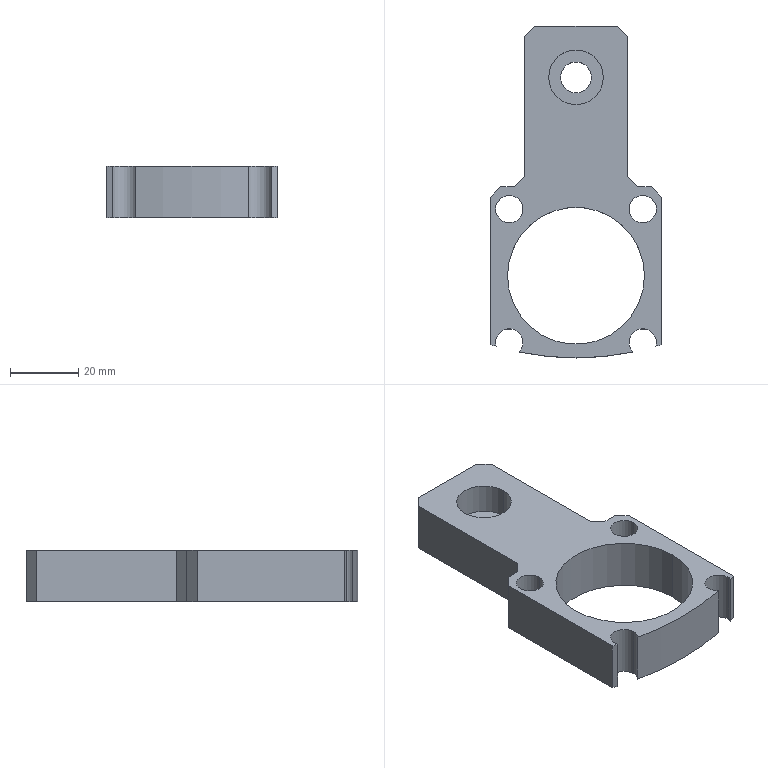Part | SolidWorks | features ICE 4, Chamfer 1, Cut 1, Extrusion 1 | 1 solid | 35 faces | box 50 x 97 x 15 mm | volume 33774 mm3 | cylinder 19 | plane 16 | commonest cylinder face diameters 8 x10 164 x3 9 x2 16 x2 40 x2
STEP:
#1=CARTESIAN_POINT('',(23.274,-3.814,15.));
#2=VERTEX_POINT('',#1);
#3=CARTESIAN_POINT('',(15.274,-3.814,15.));
#4=VERTEX_POINT('',#3);
#5=CARTESIAN_POINT('',(19.274,-3.814,15.));
#6=DIRECTION('',(0.,0.,-1.));
#7=DIRECTION('',(-1.,0.,0.));
#8=AXIS2_PLACEMENT_3D('',#5,#6,#7);
#9=CIRCLE('',#8,4.);
#10=EDGE_CURVE('',#2,#4,#9,.T.);
#11=ORIENTED_EDGE('',*,*,#10,.F.);
#12=CARTESIAN_POINT('',(23.274,-3.814,0.));
#13=VERTEX_POINT('',#12);
#14=CARTESIAN_POINT('',(23.274,-3.814,15.));
#15=DIRECTION('',(0.,0.,-1.));
#16=VECTOR('',#15,1000.);
#17=LINE('',#14,#16);
#18=EDGE_CURVE('',#2,#13,#17,.T.);
#19=ORIENTED_EDGE('',*,*,#18,.T.);
#20=CARTESIAN_POINT('',(15.274,-3.814,0.));
#21=VERTEX_POINT('',#20);
#22=CARTESIAN_POINT('',(19.274,-3.814,0.));
#23=DIRECTION('',(0.,0.,-1.));
#24=DIRECTION('',(-1.,0.,0.));
#25=AXIS2_PLACEMENT_3D('',#22,#23,#24);
#26=CIRCLE('',#25,4.);
#27=EDGE_CURVE('',#13,#21,#26,.T.);
#28=ORIENTED_EDGE('',*,*,#27,.T.);
#29=CARTESIAN_POINT('',(15.274,-3.814,15.));
#30=DIRECTION('',(0.,0.,-1.));
#31=VECTOR('',#30,1000.);
#32=LINE('',#29,#31);
#33=EDGE_CURVE('',#4,#21,#32,.T.);
#34=ORIENTED_EDGE('',*,*,#33,.F.);
#35=EDGE_LOOP('',(#11,#19,#28,#34));
#36=FACE_OUTER_BOUND('',#35,.T.);
#37=CARTESIAN_POINT('',(19.274,-3.814,15.));
#38=DIRECTION('',(0.,0.,-1.));
#39=DIRECTION('',(-1.,0.,0.));
#40=AXIS2_PLACEMENT_3D('',#37,#38,#39);
#41=CYLINDRICAL_SURFACE('',#40,4.);
#42=ADVANCED_FACE('',(#36),#41,.F.);
#43=CARTESIAN_POINT('',(-15.726,-3.814,15.));
#44=VERTEX_POINT('',#43);
#45=CARTESIAN_POINT('',(-23.726,-3.814,15.));
#46=VERTEX_POINT('',#45);
#47=CARTESIAN_POINT('',(-19.726,-3.814,15.));
#48=DIRECTION('',(0.,0.,-1.));
#49=DIRECTION('',(-1.,0.,0.));
#50=AXIS2_PLACEMENT_3D('',#47,#48,#49);
#51=CIRCLE('',#50,4.);
#52=EDGE_CURVE('',#44,#46,#51,.T.);
#53=ORIENTED_EDGE('',*,*,#52,.F.);
#54=CARTESIAN_POINT('',(-15.726,-3.814,0.));
#55=VERTEX_POINT('',#54);
#56=CARTESIAN_POINT('',(-15.726,-3.814,15.));
#57=DIRECTION('',(0.,0.,-1.));
#58=VECTOR('',#57,1000.);
#59=LINE('',#56,#58);
#60=EDGE_CURVE('',#44,#55,#59,.T.);
#61=ORIENTED_EDGE('',*,*,#60,.T.);
#62=CARTESIAN_POINT('',(-23.726,-3.814,0.));
#63=VERTEX_POINT('',#62);
#64=CARTESIAN_POINT('',(-19.726,-3.814,0.));
#65=DIRECTION('',(0.,0.,-1.));
#66=DIRECTION('',(-1.,0.,0.));
#67=AXIS2_PLACEMENT_3D('',#64,#65,#66);
#68=CIRCLE('',#67,4.);
#69=EDGE_CURVE('',#55,#63,#68,.T.);
#70=ORIENTED_EDGE('',*,*,#69,.T.);
#71=CARTESIAN_POINT('',(-23.726,-3.814,15.));
#72=DIRECTION('',(0.,0.,-1.));
#73=VECTOR('',#72,1000.);
#74=LINE('',#71,#73);
#75=EDGE_CURVE('',#46,#63,#74,.T.);
#76=ORIENTED_EDGE('',*,*,#75,.F.);
#77=EDGE_LOOP('',(#53,#61,#70,#76));
#78=FACE_OUTER_BOUND('',#77,.T.);
#79=CARTESIAN_POINT('',(-19.726,-3.814,15.));
#80=DIRECTION('',(0.,0.,-1.));
#81=DIRECTION('',(-1.,0.,0.));
#82=AXIS2_PLACEMENT_3D('',#79,#80,#81);
#83=CYLINDRICAL_SURFACE('',#82,4.);
#84=ADVANCED_FACE('',(#78),#83,.F.);
#85=CARTESIAN_POINT('',(19.774,-23.314,15.));
#86=VERTEX_POINT('',#85);
#87=CARTESIAN_POINT('',(-20.226,-23.314,15.));
#88=VERTEX_POINT('',#87);
#89=CARTESIAN_POINT('',(-0.2255,-23.314,15.));
#90=DIRECTION('',(0.,0.,-1.));
#91=DIRECTION('',(-1.,0.,0.));
#92=AXIS2_PLACEMENT_3D('',#89,#90,#91);
#93=CIRCLE('',#92,20.);
#94=EDGE_CURVE('',#86,#88,#93,.T.);
#95=ORIENTED_EDGE('',*,*,#94,.F.);
#96=CARTESIAN_POINT('',(19.774,-23.314,0.));
#97=VERTEX_POINT('',#96);
#98=CARTESIAN_POINT('',(19.774,-23.314,15.));
#99=DIRECTION('',(0.,0.,-1.));
#100=VECTOR('',#99,1000.);
#101=LINE('',#98,#100);
#102=EDGE_CURVE('',#86,#97,#101,.T.);
#103=ORIENTED_EDGE('',*,*,#102,.T.);
#104=CARTESIAN_POINT('',(-20.226,-23.314,0.));
#105=VERTEX_POINT('',#104);
#106=CARTESIAN_POINT('',(-0.2255,-23.314,0.));
#107=DIRECTION('',(0.,0.,-1.));
#108=DIRECTION('',(-1.,0.,0.));
#109=AXIS2_PLACEMENT_3D('',#106,#107,#108);
#110=CIRCLE('',#109,20.);
#111=EDGE_CURVE('',#97,#105,#110,.T.);
#112=ORIENTED_EDGE('',*,*,#111,.T.);
#113=CARTESIAN_POINT('',(-20.226,-23.314,15.));
#114=DIRECTION('',(0.,0.,-1.));
#115=VECTOR('',#114,1000.);
#116=LINE('',#113,#115);
#117=EDGE_CURVE('',#88,#105,#116,.T.);
#118=ORIENTED_EDGE('',*,*,#117,.F.);
#119=EDGE_LOOP('',(#95,#103,#112,#118));
#120=FACE_OUTER_BOUND('',#119,.T.);
#121=CARTESIAN_POINT('',(-0.2255,-23.314,15.));
#122=DIRECTION('',(0.,0.,-1.));
#123=DIRECTION('',(-1.,0.,0.));
#124=AXIS2_PLACEMENT_3D('',#121,#122,#123);
#125=CYLINDRICAL_SURFACE('',#124,20.);
#126=ADVANCED_FACE('',(#120),#125,.F.);
#127=CARTESIAN_POINT('',(-4.726,34.686,0.));
#128=VERTEX_POINT('',#127);
#129=CARTESIAN_POINT('',(4.274,34.686,0.));
#130=VERTEX_POINT('',#129);
#131=CARTESIAN_POINT('',(-0.2255,34.686,0.));
#132=DIRECTION('',(0.,0.,1.));
#133=DIRECTION('',(1.,0.,0.));
#134=AXIS2_PLACEMENT_3D('',#131,#132,#133);
#135=CIRCLE('',#134,4.5);
#136=EDGE_CURVE('',#128,#130,#135,.T.);
#137=ORIENTED_EDGE('',*,*,#136,.F.);
#138=CARTESIAN_POINT('',(-4.726,34.686,6.));
#139=VERTEX_POINT('',#138);
#140=CARTESIAN_POINT('',(-4.726,34.686,0.));
#141=DIRECTION('',(0.,0.,1.));
#142=VECTOR('',#141,1000.);
#143=LINE('',#140,#142);
#144=EDGE_CURVE('',#128,#139,#143,.T.);
#145=ORIENTED_EDGE('',*,*,#144,.T.);
#146=CARTESIAN_POINT('',(4.274,34.686,6.));
#147=VERTEX_POINT('',#146);
#148=CARTESIAN_POINT('',(-0.2255,34.686,6.));
#149=DIRECTION('',(0.,0.,1.));
#150=DIRECTION('',(1.,0.,0.));
#151=AXIS2_PLACEMENT_3D('',#148,#149,#150);
#152=CIRCLE('',#151,4.5);
#153=EDGE_CURVE('',#139,#147,#152,.T.);
#154=ORIENTED_EDGE('',*,*,#153,.T.);
#155=CARTESIAN_POINT('',(4.274,34.686,0.));
#156=DIRECTION('',(0.,0.,1.));
#157=VECTOR('',#156,1000.);
#158=LINE('',#155,#157);
#159=EDGE_CURVE('',#130,#147,#158,.T.);
#160=ORIENTED_EDGE('',*,*,#159,.F.);
#161=EDGE_LOOP('',(#137,#145,#154,#160));
#162=FACE_OUTER_BOUND('',#161,.T.);
#163=CARTESIAN_POINT('',(-0.2255,34.686,0.));
#164=DIRECTION('',(0.,0.,1.));
#165=DIRECTION('',(1.,0.,0.));
#166=AXIS2_PLACEMENT_3D('',#163,#164,#165);
#167=CYLINDRICAL_SURFACE('',#166,4.5);
#168=ADVANCED_FACE('',(#162),#167,.F.);
#169=CARTESIAN_POINT('',(-8.226,34.686,6.));
#170=VERTEX_POINT('',#169);
#171=CARTESIAN_POINT('',(7.774,34.686,6.));
#172=VERTEX_POINT('',#171);
#173=CARTESIAN_POINT('',(-0.2255,34.686,6.));
#174=DIRECTION('',(0.,0.,1.));
#175=DIRECTION('',(1.,0.,0.));
#176=AXIS2_PLACEMENT_3D('',#173,#174,#175);
#177=CIRCLE('',#176,8.);
#178=EDGE_CURVE('',#170,#172,#177,.T.);
#179=ORIENTED_EDGE('',*,*,#178,.F.);
#180=CARTESIAN_POINT('',(-8.226,34.686,15.));
#181=VERTEX_POINT('',#180);
#182=CARTESIAN_POINT('',(-8.226,34.686,6.));
#183=DIRECTION('',(0.,0.,1.));
#184=VECTOR('',#183,1000.);
#185=LINE('',#182,#184);
#186=EDGE_CURVE('',#170,#181,#185,.T.);
#187=ORIENTED_EDGE('',*,*,#186,.T.);
#188=CARTESIAN_POINT('',(7.774,34.686,15.));
#189=VERTEX_POINT('',#188);
#190=CARTESIAN_POINT('',(-0.2255,34.686,15.));
#191=DIRECTION('',(0.,0.,1.));
#192=DIRECTION('',(1.,0.,0.));
#193=AXIS2_PLACEMENT_3D('',#190,#191,#192);
#194=CIRCLE('',#193,8.);
#195=EDGE_CURVE('',#181,#189,#194,.T.);
#196=ORIENTED_EDGE('',*,*,#195,.T.);
#197=CARTESIAN_POINT('',(7.774,34.686,6.));
#198=DIRECTION('',(0.,0.,1.));
#199=VECTOR('',#198,1000.);
#200=LINE('',#197,#199);
#201=EDGE_CURVE('',#172,#189,#200,.T.);
#202=ORIENTED_EDGE('',*,*,#201,.F.);
#203=EDGE_LOOP('',(#179,#187,#196,#202));
#204=FACE_OUTER_BOUND('',#203,.T.);
#205=CARTESIAN_POINT('',(-0.2255,34.686,6.));
#206=DIRECTION('',(0.,0.,1.));
#207=DIRECTION('',(1.,0.,0.));
#208=AXIS2_PLACEMENT_3D('',#205,#206,#207);
#209=CYLINDRICAL_SURFACE('',#208,8.);
#210=ADVANCED_FACE('',(#204),#209,.F.);
#211=CARTESIAN_POINT('',(23.274,-42.814,15.));
#212=VERTEX_POINT('',#211);
#213=CARTESIAN_POINT('',(23.118,-43.922,15.));
#214=VERTEX_POINT('',#213);
#215=CARTESIAN_POINT('',(19.274,-42.814,15.));
#216=DIRECTION('',(0.,0.,-1.));
#217=DIRECTION('',(-1.,0.,0.));
#218=AXIS2_PLACEMENT_3D('',#215,#216,#217);
#219=CIRCLE('',#218,4.);
#220=EDGE_CURVE('',#212,#214,#219,.T.);
#221=ORIENTED_EDGE('',*,*,#220,.F.);
#222=CARTESIAN_POINT('',(23.274,-42.814,0.));
#223=VERTEX_POINT('',#222);
#224=CARTESIAN_POINT('',(23.274,-42.814,15.));
#225=DIRECTION('',(0.,0.,-1.));
#226=VECTOR('',#225,1000.);
#227=LINE('',#224,#226);
#228=EDGE_CURVE('',#212,#223,#227,.T.);
#229=ORIENTED_EDGE('',*,*,#228,.T.);
#230=CARTESIAN_POINT('',(23.118,-43.922,0.));
#231=VERTEX_POINT('',#230);
#232=CARTESIAN_POINT('',(19.274,-42.814,0.));
#233=DIRECTION('',(0.,0.,-1.));
#234=DIRECTION('',(-1.,0.,0.));
#235=AXIS2_PLACEMENT_3D('',#232,#233,#234);
#236=CIRCLE('',#235,4.);
#237=EDGE_CURVE('',#223,#231,#236,.T.);
#238=ORIENTED_EDGE('',*,*,#237,.T.);
#239=CARTESIAN_POINT('',(23.118,-43.922,7.5));
#240=DIRECTION('',(0.,0.,-1.));
#241=VECTOR('',#240,1000.);
#242=LINE('',#239,#241);
#243=EDGE_CURVE('',#214,#231,#242,.T.);
#244=ORIENTED_EDGE('',*,*,#243,.F.);
#245=EDGE_LOOP('',(#221,#229,#238,#244));
#246=FACE_OUTER_BOUND('',#245,.T.);
#247=CARTESIAN_POINT('',(19.274,-42.814,15.));
#248=DIRECTION('',(0.,0.,-1.));
#249=DIRECTION('',(-1.,0.,0.));
#250=AXIS2_PLACEMENT_3D('',#247,#248,#249);
#251=CYLINDRICAL_SURFACE('',#250,4.);
#252=ADVANCED_FACE('',(#246),#251,.F.);
#253=ORIENTED_EDGE('',*,*,#228,.F.);
#254=CARTESIAN_POINT('',(15.274,-42.814,15.));
#255=VERTEX_POINT('',#254);
#256=CARTESIAN_POINT('',(19.274,-42.814,15.));
#257=DIRECTION('',(0.,0.,-1.));
#258=DIRECTION('',(-1.,0.,0.));
#259=AXIS2_PLACEMENT_3D('',#256,#257,#258);
#260=CIRCLE('',#259,4.);
#261=EDGE_CURVE('',#255,#212,#260,.T.);
#262=ORIENTED_EDGE('',*,*,#261,.F.);
#263=CARTESIAN_POINT('',(15.274,-42.814,0.));
#264=VERTEX_POINT('',#263);
#265=CARTESIAN_POINT('',(15.274,-42.814,15.));
#266=DIRECTION('',(0.,0.,-1.));
#267=VECTOR('',#266,1000.);
#268=LINE('',#265,#267);
#269=EDGE_CURVE('',#255,#264,#268,.T.);
#270=ORIENTED_EDGE('',*,*,#269,.T.);
#271=CARTESIAN_POINT('',(19.274,-42.814,0.));
#272=DIRECTION('',(0.,0.,-1.));
#273=DIRECTION('',(-1.,0.,0.));
#274=AXIS2_PLACEMENT_3D('',#271,#272,#273);
#275=CIRCLE('',#274,4.);
#276=EDGE_CURVE('',#264,#223,#275,.T.);
#277=ORIENTED_EDGE('',*,*,#276,.T.);
#278=EDGE_LOOP('',(#253,#262,#270,#277));
#279=FACE_OUTER_BOUND('',#278,.T.);
#280=CARTESIAN_POINT('',(19.274,-42.814,15.));
#281=DIRECTION('',(0.,0.,-1.));
#282=DIRECTION('',(-1.,0.,0.));
#283=AXIS2_PLACEMENT_3D('',#280,#281,#282);
#284=CYLINDRICAL_SURFACE('',#283,4.);
#285=ADVANCED_FACE('',(#279),#284,.F.);
#286=CARTESIAN_POINT('',(-15.726,-42.814,15.));
#287=VERTEX_POINT('',#286);
#288=CARTESIAN_POINT('',(-16.863,-45.609,15.));
#289=VERTEX_POINT('',#288);
#290=CARTESIAN_POINT('',(-19.726,-42.814,15.));
#291=DIRECTION('',(0.,0.,-1.));
#292=DIRECTION('',(-1.,0.,0.));
#293=AXIS2_PLACEMENT_3D('',#290,#291,#292);
#294=CIRCLE('',#293,4.);
#295=EDGE_CURVE('',#287,#289,#294,.T.);
#296=ORIENTED_EDGE('',*,*,#295,.F.);
#297=CARTESIAN_POINT('',(-15.726,-42.814,0.));
#298=VERTEX_POINT('',#297);
#299=CARTESIAN_POINT('',(-15.726,-42.814,15.));
#300=DIRECTION('',(0.,0.,-1.));
#301=VECTOR('',#300,1000.);
#302=LINE('',#299,#301);
#303=EDGE_CURVE('',#287,#298,#302,.T.);
#304=ORIENTED_EDGE('',*,*,#303,.T.);
#305=CARTESIAN_POINT('',(-16.863,-45.609,0.));
#306=VERTEX_POINT('',#305);
#307=CARTESIAN_POINT('',(-19.726,-42.814,0.));
#308=DIRECTION('',(0.,0.,-1.));
#309=DIRECTION('',(-1.,0.,0.));
#310=AXIS2_PLACEMENT_3D('',#307,#308,#309);
#311=CIRCLE('',#310,4.);
#312=EDGE_CURVE('',#298,#306,#311,.T.);
#313=ORIENTED_EDGE('',*,*,#312,.T.);
#314=CARTESIAN_POINT('',(-16.863,-45.609,7.5));
#315=DIRECTION('',(0.,0.,-1.));
#316=VECTOR('',#315,1000.);
#317=LINE('',#314,#316);
#318=EDGE_CURVE('',#289,#306,#317,.T.);
#319=ORIENTED_EDGE('',*,*,#318,.F.);
#320=EDGE_LOOP('',(#296,#304,#313,#319));
#321=FACE_OUTER_BOUND('',#320,.T.);
#322=CARTESIAN_POINT('',(-19.726,-42.814,15.));
#323=DIRECTION('',(0.,0.,-1.));
#324=DIRECTION('',(-1.,0.,0.));
#325=AXIS2_PLACEMENT_3D('',#322,#323,#324);
#326=CYLINDRICAL_SURFACE('',#325,4.);
#327=ADVANCED_FACE('',(#321),#326,.F.);
#328=ORIENTED_EDGE('',*,*,#303,.F.);
#329=CARTESIAN_POINT('',(-23.726,-42.814,15.));
#330=VERTEX_POINT('',#329);
#331=CARTESIAN_POINT('',(-19.726,-42.814,15.));
#332=DIRECTION('',(0.,0.,-1.));
#333=DIRECTION('',(-1.,0.,0.));
#334=AXIS2_PLACEMENT_3D('',#331,#332,#333);
#335=CIRCLE('',#334,4.);
#336=EDGE_CURVE('',#330,#287,#335,.T.);
#337=ORIENTED_EDGE('',*,*,#336,.F.);
#338=CARTESIAN_POINT('',(-23.726,-42.814,0.));
#339=VERTEX_POINT('',#338);
#340=CARTESIAN_POINT('',(-23.726,-42.814,15.));
#341=DIRECTION('',(0.,0.,-1.));
#342=VECTOR('',#341,1000.);
#343=LINE('',#340,#342);
#344=EDGE_CURVE('',#330,#339,#343,.T.);
#345=ORIENTED_EDGE('',*,*,#344,.T.);
#346=CARTESIAN_POINT('',(-19.726,-42.814,0.));
#347=DIRECTION('',(0.,0.,-1.));
#348=DIRECTION('',(-1.,0.,0.));
#349=AXIS2_PLACEMENT_3D('',#346,#347,#348);
#350=CIRCLE('',#349,4.);
#351=EDGE_CURVE('',#339,#298,#350,.T.);
#352=ORIENTED_EDGE('',*,*,#351,.T.);
#353=EDGE_LOOP('',(#328,#337,#345,#352));
#354=FACE_OUTER_BOUND('',#353,.T.);
#355=CARTESIAN_POINT('',(-19.726,-42.814,15.));
#356=DIRECTION('',(0.,0.,-1.));
#357=DIRECTION('',(-1.,0.,0.));
#358=AXIS2_PLACEMENT_3D('',#355,#356,#357);
#359=CYLINDRICAL_SURFACE('',#358,4.);
#360=ADVANCED_FACE('',(#354),#359,.F.);
#361=CARTESIAN_POINT('',(-25.226,-43.411,15.));
#362=VERTEX_POINT('',#361);
#363=CARTESIAN_POINT('',(-25.226,-43.411,0.));
#364=VERTEX_POINT('',#363);
#365=CARTESIAN_POINT('',(-25.226,-43.411,15.));
#366=DIRECTION('',(0.,0.,-1.));
#367=VECTOR('',#366,1000.);
#368=LINE('',#365,#367);
#369=EDGE_CURVE('',#362,#364,#368,.T.);
#370=ORIENTED_EDGE('',*,*,#369,.F.);
#371=CARTESIAN_POINT('',(-25.226,-0.3145,15.));
#372=VERTEX_POINT('',#371);
#373=CARTESIAN_POINT('',(-25.226,49.686,15.));
#374=DIRECTION('',(0.,-1.,0.));
#375=VECTOR('',#374,1000.);
#376=LINE('',#373,#375);
#377=EDGE_CURVE('',#372,#362,#376,.T.);
#378=ORIENTED_EDGE('',*,*,#377,.F.);
#379=CARTESIAN_POINT('',(-25.226,-0.3145,0.));
#380=VERTEX_POINT('',#379);
#381=CARTESIAN_POINT('',(-25.226,-0.3145,15.));
#382=DIRECTION('',(0.,0.,-1.));
#383=VECTOR('',#382,1000.);
#384=LINE('',#381,#383);
#385=EDGE_CURVE('',#372,#380,#384,.T.);
#386=ORIENTED_EDGE('',*,*,#385,.T.);
#387=CARTESIAN_POINT('',(-25.226,49.686,0.));
#388=DIRECTION('',(0.,-1.,0.));
#389=VECTOR('',#388,1000.);
#390=LINE('',#387,#389);
#391=EDGE_CURVE('',#380,#364,#390,.T.);
#392=ORIENTED_EDGE('',*,*,#391,.T.);
#393=EDGE_LOOP('',(#370,#378,#386,#392));
#394=FACE_OUTER_BOUND('',#393,.T.);
#395=CARTESIAN_POINT('',(-25.226,49.686,15.));
#396=DIRECTION('',(1.,0.,0.));
#397=DIRECTION('',(0.,1.,0.));
#398=AXIS2_PLACEMENT_3D('',#395,#396,#397);
#399=PLANE('',#398);
#400=ADVANCED_FACE('',(#394),#399,.F.);
#401=CARTESIAN_POINT('',(24.774,-43.411,0.));
#402=VERTEX_POINT('',#401);
#403=CARTESIAN_POINT('',(24.774,-43.411,15.));
#404=VERTEX_POINT('',#403);
#405=CARTESIAN_POINT('',(24.774,-43.411,15.));
#406=DIRECTION('',(0.,0.,1.));
#407=VECTOR('',#406,1000.);
#408=LINE('',#405,#407);
#409=EDGE_CURVE('',#402,#404,#408,.T.);
#410=ORIENTED_EDGE('',*,*,#409,.F.);
#411=CARTESIAN_POINT('',(24.774,-0.3145,0.));
#412=VERTEX_POINT('',#411);
#413=CARTESIAN_POINT('',(24.774,49.686,0.));
#414=DIRECTION('',(0.,1.,0.));
#415=VECTOR('',#414,1000.);
#416=LINE('',#413,#415);
#417=EDGE_CURVE('',#402,#412,#416,.T.);
#418=ORIENTED_EDGE('',*,*,#417,.T.);
#419=CARTESIAN_POINT('',(24.774,-0.3145,15.));
#420=VERTEX_POINT('',#419);
#421=CARTESIAN_POINT('',(24.774,-0.3145,15.));
#422=DIRECTION('',(0.,0.,1.));
#423=VECTOR('',#422,1000.);
#424=LINE('',#421,#423);
#425=EDGE_CURVE('',#412,#420,#424,.T.);
#426=ORIENTED_EDGE('',*,*,#425,.T.);
#427=CARTESIAN_POINT('',(24.774,49.686,15.));
#428=DIRECTION('',(0.,1.,0.));
#429=VECTOR('',#428,1000.);
#430=LINE('',#427,#429);
#431=EDGE_CURVE('',#404,#420,#430,.T.);
#432=ORIENTED_EDGE('',*,*,#431,.F.);
#433=EDGE_LOOP('',(#410,#418,#426,#432));
#434=FACE_OUTER_BOUND('',#433,.T.);
#435=CARTESIAN_POINT('',(24.774,49.686,15.));
#436=DIRECTION('',(-1.,0.,0.));
#437=DIRECTION('',(0.,-1.,0.));
#438=AXIS2_PLACEMENT_3D('',#435,#436,#437);
#439=PLANE('',#438);
#440=ADVANCED_FACE('',(#434),#439,.F.);
#441=CARTESIAN_POINT('',(19.274,-3.814,15.));
#442=DIRECTION('',(0.,0.,-1.));
#443=DIRECTION('',(-1.,0.,0.));
#444=AXIS2_PLACEMENT_3D('',#441,#442,#443);
#445=CIRCLE('',#444,4.);
#446=EDGE_CURVE('',#4,#2,#445,.T.);
#447=ORIENTED_EDGE('',*,*,#446,.T.);
#448=ORIENTED_EDGE('',*,*,#10,.T.);
#449=EDGE_LOOP('',(#447,#448));
#450=FACE_BOUND('',#449,.T.);
#451=CARTESIAN_POINT('',(-19.726,-3.814,15.));
#452=DIRECTION('',(0.,0.,-1.));
#453=DIRECTION('',(-1.,0.,0.));
#454=AXIS2_PLACEMENT_3D('',#451,#452,#453);
#455=CIRCLE('',#454,4.);
#456=EDGE_CURVE('',#46,#44,#455,.T.);
#457=ORIENTED_EDGE('',*,*,#456,.T.);
#458=ORIENTED_EDGE('',*,*,#52,.T.);
#459=EDGE_LOOP('',(#457,#458));
#460=FACE_BOUND('',#459,.T.);
#461=CARTESIAN_POINT('',(-0.2255,-23.314,15.));
#462=DIRECTION('',(0.,0.,-1.));
#463=DIRECTION('',(-1.,0.,0.));
#464=AXIS2_PLACEMENT_3D('',#461,#462,#463);
#465=CIRCLE('',#464,20.);
#466=EDGE_CURVE('',#88,#86,#465,.T.);
#467=ORIENTED_EDGE('',*,*,#466,.T.);
#468=ORIENTED_EDGE('',*,*,#94,.T.);
#469=EDGE_LOOP('',(#467,#468));
#470=FACE_BOUND('',#469,.T.);
#471=CARTESIAN_POINT('',(-0.2255,34.686,15.));
#472=DIRECTION('',(0.,0.,1.));
#473=DIRECTION('',(1.,0.,0.));
#474=AXIS2_PLACEMENT_3D('',#471,#472,#473);
#475=CIRCLE('',#474,8.);
#476=EDGE_CURVE('',#189,#181,#475,.T.);
#477=ORIENTED_EDGE('',*,*,#476,.F.);
#478=ORIENTED_EDGE('',*,*,#195,.F.);
#479=EDGE_LOOP('',(#477,#478));
#480=FACE_BOUND('',#479,.T.);
#481=ORIENTED_EDGE('',*,*,#377,.T.);
#482=CARTESIAN_POINT('',(-23.569,-43.922,15.));
#483=VERTEX_POINT('',#482);
#484=CARTESIAN_POINT('',(-0.2255,34.686,15.));
#485=DIRECTION('',(0.,0.,-1.));
#486=DIRECTION('',(-1.,0.,0.));
#487=AXIS2_PLACEMENT_3D('',#484,#485,#486);
#488=CIRCLE('',#487,82.);
#489=EDGE_CURVE('',#483,#362,#488,.T.);
#490=ORIENTED_EDGE('',*,*,#489,.F.);
#491=CARTESIAN_POINT('',(-19.726,-42.814,15.));
#492=DIRECTION('',(0.,0.,-1.));
#493=DIRECTION('',(-1.,0.,0.));
#494=AXIS2_PLACEMENT_3D('',#491,#492,#493);
#495=CIRCLE('',#494,4.);
#496=EDGE_CURVE('',#483,#330,#495,.T.);
#497=ORIENTED_EDGE('',*,*,#496,.T.);
#498=ORIENTED_EDGE('',*,*,#336,.T.);
#499=ORIENTED_EDGE('',*,*,#295,.T.);
#500=CARTESIAN_POINT('',(16.412,-45.609,15.));
#501=VERTEX_POINT('',#500);
#502=CARTESIAN_POINT('',(-0.2255,34.686,15.));
#503=DIRECTION('',(0.,0.,-1.));
#504=DIRECTION('',(-1.,0.,0.));
#505=AXIS2_PLACEMENT_3D('',#502,#503,#504);
#506=CIRCLE('',#505,82.);
#507=EDGE_CURVE('',#501,#289,#506,.T.);
#508=ORIENTED_EDGE('',*,*,#507,.F.);
#509=CARTESIAN_POINT('',(19.274,-42.814,15.));
#510=DIRECTION('',(0.,0.,-1.));
#511=DIRECTION('',(-1.,0.,0.));
#512=AXIS2_PLACEMENT_3D('',#509,#510,#511);
#513=CIRCLE('',#512,4.);
#514=EDGE_CURVE('',#501,#255,#513,.T.);
#515=ORIENTED_EDGE('',*,*,#514,.T.);
#516=ORIENTED_EDGE('',*,*,#261,.T.);
#517=ORIENTED_EDGE('',*,*,#220,.T.);
#518=CARTESIAN_POINT('',(-0.2255,34.686,15.));
#519=DIRECTION('',(0.,0.,-1.));
#520=DIRECTION('',(-1.,0.,0.));
#521=AXIS2_PLACEMENT_3D('',#518,#519,#520);
#522=CIRCLE('',#521,82.);
#523=EDGE_CURVE('',#404,#214,#522,.T.);
#524=ORIENTED_EDGE('',*,*,#523,.F.);
#525=ORIENTED_EDGE('',*,*,#431,.T.);
#526=CARTESIAN_POINT('',(21.774,2.686,15.));
#527=VERTEX_POINT('',#526);
#528=CARTESIAN_POINT('',(12.23,12.23,15.));
#529=DIRECTION('',(-0.7071,0.7071,0.));
#530=VECTOR('',#529,1000.);
#531=LINE('',#528,#530);
#532=EDGE_CURVE('',#420,#527,#531,.T.);
#533=ORIENTED_EDGE('',*,*,#532,.T.);
#534=CARTESIAN_POINT('',(17.774,2.686,15.));
#535=VERTEX_POINT('',#534);
#536=CARTESIAN_POINT('',(14.774,2.686,15.));
#537=DIRECTION('',(1.,0.,0.));
#538=VECTOR('',#537,1000.);
#539=LINE('',#536,#538);
#540=EDGE_CURVE('',#535,#527,#539,.T.);
#541=ORIENTED_EDGE('',*,*,#540,.F.);
#542=CARTESIAN_POINT('',(14.774,5.686,15.));
#543=VERTEX_POINT('',#542);
#544=CARTESIAN_POINT('',(17.774,2.686,15.));
#545=DIRECTION('',(-0.7071,0.7071,0.));
#546=VECTOR('',#545,1000.);
#547=LINE('',#544,#546);
#548=EDGE_CURVE('',#535,#543,#547,.T.);
#549=ORIENTED_EDGE('',*,*,#548,.T.);
#550=CARTESIAN_POINT('',(14.774,46.686,15.));
#551=VERTEX_POINT('',#550);
#552=CARTESIAN_POINT('',(14.774,64.722,15.));
#553=DIRECTION('',(0.,-1.,0.));
#554=VECTOR('',#553,1000.);
#555=LINE('',#552,#554);
#556=EDGE_CURVE('',#551,#543,#555,.T.);
#557=ORIENTED_EDGE('',*,*,#556,.F.);
#558=CARTESIAN_POINT('',(11.774,49.686,15.));
#559=VERTEX_POINT('',#558);
#560=CARTESIAN_POINT('',(30.73,30.73,15.));
#561=DIRECTION('',(-0.7071,0.7071,0.));
#562=VECTOR('',#561,1000.);
#563=LINE('',#560,#562);
#564=EDGE_CURVE('',#551,#559,#563,.T.);
#565=ORIENTED_EDGE('',*,*,#564,.T.);
#566=CARTESIAN_POINT('',(-12.226,49.686,15.));
#567=VERTEX_POINT('',#566);
#568=CARTESIAN_POINT('',(-25.226,49.686,15.));
#569=DIRECTION('',(-1.,0.,0.));
#570=VECTOR('',#569,1000.);
#571=LINE('',#568,#570);
#572=EDGE_CURVE('',#559,#567,#571,.T.);
#573=ORIENTED_EDGE('',*,*,#572,.T.);
#574=CARTESIAN_POINT('',(-15.226,46.686,15.));
#575=VERTEX_POINT('',#574);
#576=CARTESIAN_POINT('',(-30.956,30.956,15.));
#577=DIRECTION('',(-0.7071,-0.7071,0.));
#578=VECTOR('',#577,1000.);
#579=LINE('',#576,#578);
#580=EDGE_CURVE('',#567,#575,#579,.T.);
#581=ORIENTED_EDGE('',*,*,#580,.T.);
#582=CARTESIAN_POINT('',(-15.226,5.686,15.));
#583=VERTEX_POINT('',#582);
#584=CARTESIAN_POINT('',(-15.226,55.257,15.));
#585=DIRECTION('',(0.,1.,0.));
#586=VECTOR('',#585,1000.);
#587=LINE('',#584,#586);
#588=EDGE_CURVE('',#583,#575,#587,.T.);
#589=ORIENTED_EDGE('',*,*,#588,.F.);
#590=CARTESIAN_POINT('',(-18.226,2.686,15.));
#591=VERTEX_POINT('',#590);
#592=CARTESIAN_POINT('',(-15.226,5.686,15.));
#593=DIRECTION('',(-0.7071,-0.7071,0.));
#594=VECTOR('',#593,1000.);
#595=LINE('',#592,#594);
#596=EDGE_CURVE('',#583,#591,#595,.T.);
#597=ORIENTED_EDGE('',*,*,#596,.T.);
#598=CARTESIAN_POINT('',(-22.226,2.686,15.));
#599=VERTEX_POINT('',#598);
#600=CARTESIAN_POINT('',(-15.226,2.686,15.));
#601=DIRECTION('',(1.,0.,0.));
#602=VECTOR('',#601,1000.);
#603=LINE('',#600,#602);
#604=EDGE_CURVE('',#599,#591,#603,.T.);
#605=ORIENTED_EDGE('',*,*,#604,.F.);
#606=CARTESIAN_POINT('',(-12.456,12.456,15.));
#607=DIRECTION('',(-0.7071,-0.7071,0.));
#608=VECTOR('',#607,1000.);
#609=LINE('',#606,#608);
#610=EDGE_CURVE('',#599,#372,#609,.T.);
#611=ORIENTED_EDGE('',*,*,#610,.T.);
#612=EDGE_LOOP('',(#481,#490,#497,#498,#499,#508,#515,#516,#517,#524,#525,#533,#541,#549,#557,#565,#573,#581,#589,#597,#605,#611));
#613=FACE_OUTER_BOUND('',#612,.T.);
#614=CARTESIAN_POINT('',(0.,0.,15.));
#615=DIRECTION('',(0.,0.,1.));
#616=DIRECTION('',(1.,0.,0.));
#617=AXIS2_PLACEMENT_3D('',#614,#615,#616);
#618=PLANE('',#617);
#619=ADVANCED_FACE('',(#450,#460,#470,#480,#613),#618,.T.);
#620=CARTESIAN_POINT('',(19.274,-3.814,0.));
#621=DIRECTION('',(0.,0.,-1.));
#622=DIRECTION('',(-1.,0.,0.));
#623=AXIS2_PLACEMENT_3D('',#620,#621,#622);
#624=CIRCLE('',#623,4.);
#625=EDGE_CURVE('',#21,#13,#624,.T.);
#626=ORIENTED_EDGE('',*,*,#625,.F.);
#627=ORIENTED_EDGE('',*,*,#27,.F.);
#628=EDGE_LOOP('',(#626,#627));
#629=FACE_BOUND('',#628,.T.);
#630=CARTESIAN_POINT('',(-19.726,-3.814,0.));
#631=DIRECTION('',(0.,0.,-1.));
#632=DIRECTION('',(-1.,0.,0.));
#633=AXIS2_PLACEMENT_3D('',#630,#631,#632);
#634=CIRCLE('',#633,4.);
#635=EDGE_CURVE('',#63,#55,#634,.T.);
#636=ORIENTED_EDGE('',*,*,#635,.F.);
#637=ORIENTED_EDGE('',*,*,#69,.F.);
#638=EDGE_LOOP('',(#636,#637));
#639=FACE_BOUND('',#638,.T.);
#640=CARTESIAN_POINT('',(-0.2255,-23.314,0.));
#641=DIRECTION('',(0.,0.,-1.));
#642=DIRECTION('',(-1.,0.,0.));
#643=AXIS2_PLACEMENT_3D('',#640,#641,#642);
#644=CIRCLE('',#643,20.);
#645=EDGE_CURVE('',#105,#97,#644,.T.);
#646=ORIENTED_EDGE('',*,*,#645,.F.);
#647=ORIENTED_EDGE('',*,*,#111,.F.);
#648=EDGE_LOOP('',(#646,#647));
#649=FACE_BOUND('',#648,.T.);
#650=CARTESIAN_POINT('',(-0.2255,34.686,0.));
#651=DIRECTION('',(0.,0.,1.));
#652=DIRECTION('',(1.,0.,0.));
#653=AXIS2_PLACEMENT_3D('',#650,#651,#652);
#654=CIRCLE('',#653,4.5);
#655=EDGE_CURVE('',#130,#128,#654,.T.);
#656=ORIENTED_EDGE('',*,*,#655,.T.);
#657=ORIENTED_EDGE('',*,*,#136,.T.);
#658=EDGE_LOOP('',(#656,#657));
#659=FACE_BOUND('',#658,.T.);
#660=CARTESIAN_POINT('',(-23.569,-43.922,0.));
#661=VERTEX_POINT('',#660);
#662=CARTESIAN_POINT('',(-0.2255,34.686,0.));
#663=DIRECTION('',(0.,0.,-1.));
#664=DIRECTION('',(-1.,0.,0.));
#665=AXIS2_PLACEMENT_3D('',#662,#663,#664);
#666=CIRCLE('',#665,82.);
#667=EDGE_CURVE('',#661,#364,#666,.T.);
#668=ORIENTED_EDGE('',*,*,#667,.T.);
#669=ORIENTED_EDGE('',*,*,#391,.F.);
#670=CARTESIAN_POINT('',(-22.226,2.686,0.));
#671=VERTEX_POINT('',#670);
#672=CARTESIAN_POINT('',(-25.226,-0.3145,0.));
#673=DIRECTION('',(0.7071,0.7071,0.));
#674=VECTOR('',#673,1000.);
#675=LINE('',#672,#674);
#676=EDGE_CURVE('',#380,#671,#675,.T.);
#677=ORIENTED_EDGE('',*,*,#676,.T.);
#678=CARTESIAN_POINT('',(-18.226,2.686,0.));
#679=VERTEX_POINT('',#678);
#680=CARTESIAN_POINT('',(0.,2.686,0.));
#681=DIRECTION('',(1.,0.,0.));
#682=VECTOR('',#681,1000.);
#683=LINE('',#680,#682);
#684=EDGE_CURVE('',#671,#679,#683,.T.);
#685=ORIENTED_EDGE('',*,*,#684,.T.);
#686=CARTESIAN_POINT('',(-15.226,5.686,0.));
#687=VERTEX_POINT('',#686);
#688=CARTESIAN_POINT('',(-10.456,10.456,0.));
#689=DIRECTION('',(0.7071,0.7071,0.));
#690=VECTOR('',#689,1000.);
#691=LINE('',#688,#690);
#692=EDGE_CURVE('',#679,#687,#691,.T.);
#693=ORIENTED_EDGE('',*,*,#692,.T.);
#694=CARTESIAN_POINT('',(-15.226,46.686,0.));
#695=VERTEX_POINT('',#694);
#696=CARTESIAN_POINT('',(-15.226,55.257,0.));
#697=DIRECTION('',(0.,1.,0.));
#698=VECTOR('',#697,1000.);
#699=LINE('',#696,#698);
#700=EDGE_CURVE('',#687,#695,#699,.T.);
#701=ORIENTED_EDGE('',*,*,#700,.T.);
#702=CARTESIAN_POINT('',(-12.226,49.686,0.));
#703=VERTEX_POINT('',#702);
#704=CARTESIAN_POINT('',(-12.226,49.686,0.));
#705=DIRECTION('',(0.7071,0.7071,0.));
#706=VECTOR('',#705,1000.);
#707=LINE('',#704,#706);
#708=EDGE_CURVE('',#695,#703,#707,.T.);
#709=ORIENTED_EDGE('',*,*,#708,.T.);
#710=CARTESIAN_POINT('',(11.774,49.686,0.));
#711=VERTEX_POINT('',#710);
#712=CARTESIAN_POINT('',(-25.226,49.686,0.));
#713=DIRECTION('',(-1.,0.,0.));
#714=VECTOR('',#713,1000.);
#715=LINE('',#712,#714);
#716=EDGE_CURVE('',#711,#703,#715,.T.);
#717=ORIENTED_EDGE('',*,*,#716,.F.);
#718=CARTESIAN_POINT('',(14.774,46.686,0.));
#719=VERTEX_POINT('',#718);
#720=CARTESIAN_POINT('',(11.774,49.686,0.));
#721=DIRECTION('',(0.7071,-0.7071,0.));
#722=VECTOR('',#721,1000.);
#723=LINE('',#720,#722);
#724=EDGE_CURVE('',#711,#719,#723,.T.);
#725=ORIENTED_EDGE('',*,*,#724,.T.);
#726=CARTESIAN_POINT('',(14.774,5.686,0.));
#727=VERTEX_POINT('',#726);
#728=CARTESIAN_POINT('',(14.774,0.,0.));
#729=DIRECTION('',(0.,-1.,0.));
#730=VECTOR('',#729,1000.);
#731=LINE('',#728,#730);
#732=EDGE_CURVE('',#719,#727,#731,.T.);
#733=ORIENTED_EDGE('',*,*,#732,.T.);
#734=CARTESIAN_POINT('',(17.774,2.686,0.));
#735=VERTEX_POINT('',#734);
#736=CARTESIAN_POINT('',(10.23,10.23,0.));
#737=DIRECTION('',(0.7071,-0.7071,0.));
#738=VECTOR('',#737,1000.);
#739=LINE('',#736,#738);
#740=EDGE_CURVE('',#727,#735,#739,.T.);
#741=ORIENTED_EDGE('',*,*,#740,.T.);
#742=CARTESIAN_POINT('',(21.774,2.686,0.));
#743=VERTEX_POINT('',#742);
#744=CARTESIAN_POINT('',(14.774,2.686,0.));
#745=DIRECTION('',(1.,0.,0.));
#746=VECTOR('',#745,1000.);
#747=LINE('',#744,#746);
#748=EDGE_CURVE('',#735,#743,#747,.T.);
#749=ORIENTED_EDGE('',*,*,#748,.T.);
#750=CARTESIAN_POINT('',(24.774,-0.3145,0.));
#751=DIRECTION('',(0.7071,-0.7071,0.));
#752=VECTOR('',#751,1000.);
#753=LINE('',#750,#752);
#754=EDGE_CURVE('',#743,#412,#753,.T.);
#755=ORIENTED_EDGE('',*,*,#754,.T.);
#756=ORIENTED_EDGE('',*,*,#417,.F.);
#757=CARTESIAN_POINT('',(-0.2255,34.686,0.));
#758=DIRECTION('',(0.,0.,-1.));
#759=DIRECTION('',(-1.,0.,0.));
#760=AXIS2_PLACEMENT_3D('',#757,#758,#759);
#761=CIRCLE('',#760,82.);
#762=EDGE_CURVE('',#402,#231,#761,.T.);
#763=ORIENTED_EDGE('',*,*,#762,.T.);
#764=ORIENTED_EDGE('',*,*,#237,.F.);
#765=ORIENTED_EDGE('',*,*,#276,.F.);
#766=CARTESIAN_POINT('',(16.412,-45.609,0.));
#767=VERTEX_POINT('',#766);
#768=CARTESIAN_POINT('',(19.274,-42.814,0.));
#769=DIRECTION('',(0.,0.,-1.));
#770=DIRECTION('',(-1.,0.,0.));
#771=AXIS2_PLACEMENT_3D('',#768,#769,#770);
#772=CIRCLE('',#771,4.);
#773=EDGE_CURVE('',#767,#264,#772,.T.);
#774=ORIENTED_EDGE('',*,*,#773,.F.);
#775=CARTESIAN_POINT('',(-0.2255,34.686,0.));
#776=DIRECTION('',(0.,0.,-1.));
#777=DIRECTION('',(-1.,0.,0.));
#778=AXIS2_PLACEMENT_3D('',#775,#776,#777);
#779=CIRCLE('',#778,82.);
#780=EDGE_CURVE('',#767,#306,#779,.T.);
#781=ORIENTED_EDGE('',*,*,#780,.T.);
#782=ORIENTED_EDGE('',*,*,#312,.F.);
#783=ORIENTED_EDGE('',*,*,#351,.F.);
#784=CARTESIAN_POINT('',(-19.726,-42.814,0.));
#785=DIRECTION('',(0.,0.,-1.));
#786=DIRECTION('',(-1.,0.,0.));
#787=AXIS2_PLACEMENT_3D('',#784,#785,#786);
#788=CIRCLE('',#787,4.);
#789=EDGE_CURVE('',#661,#339,#788,.T.);
#790=ORIENTED_EDGE('',*,*,#789,.F.);
#791=EDGE_LOOP('',(#668,#669,#677,#685,#693,#701,#709,#717,#725,#733,#741,#749,#755,#756,#763,#764,#765,#774,#781,#782,#783,#790));
#792=FACE_OUTER_BOUND('',#791,.T.);
#793=CARTESIAN_POINT('',(0.,0.,0.));
#794=DIRECTION('',(0.,0.,1.));
#795=DIRECTION('',(1.,0.,0.));
#796=AXIS2_PLACEMENT_3D('',#793,#794,#795);
#797=PLANE('',#796);
#798=ADVANCED_FACE('',(#629,#639,#649,#659,#792),#797,.F.);
#799=ORIENTED_EDGE('',*,*,#344,.F.);
#800=ORIENTED_EDGE('',*,*,#496,.F.);
#801=CARTESIAN_POINT('',(-23.569,-43.922,7.5));
#802=DIRECTION('',(0.,0.,1.));
#803=VECTOR('',#802,1000.);
#804=LINE('',#801,#803);
#805=EDGE_CURVE('',#661,#483,#804,.T.);
#806=ORIENTED_EDGE('',*,*,#805,.F.);
#807=ORIENTED_EDGE('',*,*,#789,.T.);
#808=EDGE_LOOP('',(#799,#800,#806,#807));
#809=FACE_OUTER_BOUND('',#808,.T.);
#810=CARTESIAN_POINT('',(-19.726,-42.814,15.));
#811=DIRECTION('',(0.,0.,-1.));
#812=DIRECTION('',(-1.,0.,0.));
#813=AXIS2_PLACEMENT_3D('',#810,#811,#812);
#814=CYLINDRICAL_SURFACE('',#813,4.);
#815=ADVANCED_FACE('',(#809),#814,.F.);
#816=ORIENTED_EDGE('',*,*,#269,.F.);
#817=ORIENTED_EDGE('',*,*,#514,.F.);
#818=CARTESIAN_POINT('',(16.412,-45.609,7.5));
#819=DIRECTION('',(0.,0.,1.));
#820=VECTOR('',#819,1000.);
#821=LINE('',#818,#820);
#822=EDGE_CURVE('',#767,#501,#821,.T.);
#823=ORIENTED_EDGE('',*,*,#822,.F.);
#824=ORIENTED_EDGE('',*,*,#773,.T.);
#825=EDGE_LOOP('',(#816,#817,#823,#824));
#826=FACE_OUTER_BOUND('',#825,.T.);
#827=CARTESIAN_POINT('',(19.274,-42.814,15.));
#828=DIRECTION('',(0.,0.,-1.));
#829=DIRECTION('',(-1.,0.,0.));
#830=AXIS2_PLACEMENT_3D('',#827,#828,#829);
#831=CYLINDRICAL_SURFACE('',#830,4.);
#832=ADVANCED_FACE('',(#826),#831,.F.);
#833=ORIENTED_EDGE('',*,*,#572,.F.);
#834=CARTESIAN_POINT('',(11.774,49.686,15.));
#835=DIRECTION('',(0.,0.,-1.));
#836=VECTOR('',#835,1000.);
#837=LINE('',#834,#836);
#838=EDGE_CURVE('',#559,#711,#837,.T.);
#839=ORIENTED_EDGE('',*,*,#838,.T.);
#840=ORIENTED_EDGE('',*,*,#716,.T.);
#841=CARTESIAN_POINT('',(-12.226,49.686,15.));
#842=DIRECTION('',(0.,0.,1.));
#843=VECTOR('',#842,1000.);
#844=LINE('',#841,#843);
#845=EDGE_CURVE('',#703,#567,#844,.T.);
#846=ORIENTED_EDGE('',*,*,#845,.T.);
#847=EDGE_LOOP('',(#833,#839,#840,#846));
#848=FACE_OUTER_BOUND('',#847,.T.);
#849=CARTESIAN_POINT('',(-25.226,49.686,15.));
#850=DIRECTION('',(0.,-1.,0.));
#851=DIRECTION('',(0.,0.,-1.));
#852=AXIS2_PLACEMENT_3D('',#849,#850,#851);
#853=PLANE('',#852);
#854=ADVANCED_FACE('',(#848),#853,.F.);
#855=ORIENTED_EDGE('',*,*,#186,.F.);
#856=CARTESIAN_POINT('',(-0.2255,34.686,6.));
#857=DIRECTION('',(0.,0.,1.));
#858=DIRECTION('',(1.,0.,0.));
#859=AXIS2_PLACEMENT_3D('',#856,#857,#858);
#860=CIRCLE('',#859,8.);
#861=EDGE_CURVE('',#172,#170,#860,.T.);
#862=ORIENTED_EDGE('',*,*,#861,.F.);
#863=ORIENTED_EDGE('',*,*,#201,.T.);
#864=ORIENTED_EDGE('',*,*,#476,.T.);
#865=EDGE_LOOP('',(#855,#862,#863,#864));
#866=FACE_OUTER_BOUND('',#865,.T.);
#867=CARTESIAN_POINT('',(-0.2255,34.686,6.));
#868=DIRECTION('',(0.,0.,1.));
#869=DIRECTION('',(1.,0.,0.));
#870=AXIS2_PLACEMENT_3D('',#867,#868,#869);
#871=CYLINDRICAL_SURFACE('',#870,8.);
#872=ADVANCED_FACE('',(#866),#871,.F.);
#873=CARTESIAN_POINT('',(-0.2255,34.686,6.));
#874=DIRECTION('',(0.,0.,1.));
#875=DIRECTION('',(1.,0.,0.));
#876=AXIS2_PLACEMENT_3D('',#873,#874,#875);
#877=CIRCLE('',#876,4.5);
#878=EDGE_CURVE('',#147,#139,#877,.T.);
#879=ORIENTED_EDGE('',*,*,#878,.F.);
#880=ORIENTED_EDGE('',*,*,#153,.F.);
#881=EDGE_LOOP('',(#879,#880));
#882=FACE_BOUND('',#881,.T.);
#883=ORIENTED_EDGE('',*,*,#861,.T.);
#884=ORIENTED_EDGE('',*,*,#178,.T.);
#885=EDGE_LOOP('',(#883,#884));
#886=FACE_OUTER_BOUND('',#885,.T.);
#887=CARTESIAN_POINT('',(-0.2255,34.686,6.));
#888=DIRECTION('',(0.,0.,1.));
#889=DIRECTION('',(1.,0.,0.));
#890=AXIS2_PLACEMENT_3D('',#887,#888,#889);
#891=PLANE('',#890);
#892=ADVANCED_FACE('',(#882,#886),#891,.T.);
#893=ORIENTED_EDGE('',*,*,#144,.F.);
#894=ORIENTED_EDGE('',*,*,#655,.F.);
#895=ORIENTED_EDGE('',*,*,#159,.T.);
#896=ORIENTED_EDGE('',*,*,#878,.T.);
#897=EDGE_LOOP('',(#893,#894,#895,#896));
#898=FACE_OUTER_BOUND('',#897,.T.);
#899=CARTESIAN_POINT('',(-0.2255,34.686,0.));
#900=DIRECTION('',(0.,0.,1.));
#901=DIRECTION('',(1.,0.,0.));
#902=AXIS2_PLACEMENT_3D('',#899,#900,#901);
#903=CYLINDRICAL_SURFACE('',#902,4.5);
#904=ADVANCED_FACE('',(#898),#903,.F.);
#905=ORIENTED_EDGE('',*,*,#102,.F.);
#906=ORIENTED_EDGE('',*,*,#466,.F.);
#907=ORIENTED_EDGE('',*,*,#117,.T.);
#908=ORIENTED_EDGE('',*,*,#645,.T.);
#909=EDGE_LOOP('',(#905,#906,#907,#908));
#910=FACE_OUTER_BOUND('',#909,.T.);
#911=CARTESIAN_POINT('',(-0.2255,-23.314,15.));
#912=DIRECTION('',(0.,0.,-1.));
#913=DIRECTION('',(-1.,0.,0.));
#914=AXIS2_PLACEMENT_3D('',#911,#912,#913);
#915=CYLINDRICAL_SURFACE('',#914,20.);
#916=ADVANCED_FACE('',(#910),#915,.F.);
#917=ORIENTED_EDGE('',*,*,#60,.F.);
#918=ORIENTED_EDGE('',*,*,#456,.F.);
#919=ORIENTED_EDGE('',*,*,#75,.T.);
#920=ORIENTED_EDGE('',*,*,#635,.T.);
#921=EDGE_LOOP('',(#917,#918,#919,#920));
#922=FACE_OUTER_BOUND('',#921,.T.);
#923=CARTESIAN_POINT('',(-19.726,-3.814,15.));
#924=DIRECTION('',(0.,0.,-1.));
#925=DIRECTION('',(-1.,0.,0.));
#926=AXIS2_PLACEMENT_3D('',#923,#924,#925);
#927=CYLINDRICAL_SURFACE('',#926,4.);
#928=ADVANCED_FACE('',(#922),#927,.F.);
#929=ORIENTED_EDGE('',*,*,#18,.F.);
#930=ORIENTED_EDGE('',*,*,#446,.F.);
#931=ORIENTED_EDGE('',*,*,#33,.T.);
#932=ORIENTED_EDGE('',*,*,#625,.T.);
#933=EDGE_LOOP('',(#929,#930,#931,#932));
#934=FACE_OUTER_BOUND('',#933,.T.);
#935=CARTESIAN_POINT('',(19.274,-3.814,15.));
#936=DIRECTION('',(0.,0.,-1.));
#937=DIRECTION('',(-1.,0.,0.));
#938=AXIS2_PLACEMENT_3D('',#935,#936,#937);
#939=CYLINDRICAL_SURFACE('',#938,4.);
#940=ADVANCED_FACE('',(#934),#939,.F.);
#941=ORIENTED_EDGE('',*,*,#556,.T.);
#942=CARTESIAN_POINT('',(14.774,5.686,0.));
#943=DIRECTION('',(0.,0.,-1.));
#944=VECTOR('',#943,1000.);
#945=LINE('',#942,#944);
#946=EDGE_CURVE('',#543,#727,#945,.T.);
#947=ORIENTED_EDGE('',*,*,#946,.T.);
#948=ORIENTED_EDGE('',*,*,#732,.F.);
#949=CARTESIAN_POINT('',(14.774,46.686,0.));
#950=DIRECTION('',(0.,0.,1.));
#951=VECTOR('',#950,1000.);
#952=LINE('',#949,#951);
#953=EDGE_CURVE('',#719,#551,#952,.T.);
#954=ORIENTED_EDGE('',*,*,#953,.T.);
#955=EDGE_LOOP('',(#941,#947,#948,#954));
#956=FACE_OUTER_BOUND('',#955,.T.);
#957=CARTESIAN_POINT('',(14.774,64.722,0.));
#958=DIRECTION('',(-1.,0.,0.));
#959=DIRECTION('',(0.,-1.,0.));
#960=AXIS2_PLACEMENT_3D('',#957,#958,#959);
#961=PLANE('',#960);
#962=ADVANCED_FACE('',(#956),#961,.F.);
#963=ORIENTED_EDGE('',*,*,#748,.F.);
#964=CARTESIAN_POINT('',(17.774,2.686,15.));
#965=DIRECTION('',(0.,0.,1.));
#966=VECTOR('',#965,1000.);
#967=LINE('',#964,#966);
#968=EDGE_CURVE('',#735,#535,#967,.T.);
#969=ORIENTED_EDGE('',*,*,#968,.T.);
#970=ORIENTED_EDGE('',*,*,#540,.T.);
#971=CARTESIAN_POINT('',(21.774,2.686,0.));
#972=DIRECTION('',(0.,0.,-1.));
#973=VECTOR('',#972,1000.);
#974=LINE('',#971,#973);
#975=EDGE_CURVE('',#527,#743,#974,.T.);
#976=ORIENTED_EDGE('',*,*,#975,.T.);
#977=EDGE_LOOP('',(#963,#969,#970,#976));
#978=FACE_OUTER_BOUND('',#977,.T.);
#979=CARTESIAN_POINT('',(14.774,2.686,0.));
#980=DIRECTION('',(0.,-1.,0.));
#981=DIRECTION('',(0.,0.,-1.));
#982=AXIS2_PLACEMENT_3D('',#979,#980,#981);
#983=PLANE('',#982);
#984=ADVANCED_FACE('',(#978),#983,.F.);
#985=ORIENTED_EDGE('',*,*,#700,.F.);
#986=CARTESIAN_POINT('',(-15.226,5.686,15.));
#987=DIRECTION('',(0.,0.,1.));
#988=VECTOR('',#987,1000.);
#989=LINE('',#986,#988);
#990=EDGE_CURVE('',#687,#583,#989,.T.);
#991=ORIENTED_EDGE('',*,*,#990,.T.);
#992=ORIENTED_EDGE('',*,*,#588,.T.);
#993=CARTESIAN_POINT('',(-15.226,46.686,0.));
#994=DIRECTION('',(0.,0.,-1.));
#995=VECTOR('',#994,1000.);
#996=LINE('',#993,#995);
#997=EDGE_CURVE('',#575,#695,#996,.T.);
#998=ORIENTED_EDGE('',*,*,#997,.T.);
#999=EDGE_LOOP('',(#985,#991,#992,#998));
#1000=FACE_OUTER_BOUND('',#999,.T.);
#1001=CARTESIAN_POINT('',(-15.226,55.257,0.));
#1002=DIRECTION('',(1.,0.,0.));
#1003=DIRECTION('',(0.,1.,0.));
#1004=AXIS2_PLACEMENT_3D('',#1001,#1002,#1003);
#1005=PLANE('',#1004);
#1006=ADVANCED_FACE('',(#1000),#1005,.F.);
#1007=ORIENTED_EDGE('',*,*,#604,.T.);
#1008=CARTESIAN_POINT('',(-18.226,2.686,0.));
#1009=DIRECTION('',(0.,0.,-1.));
#1010=VECTOR('',#1009,1000.);
#1011=LINE('',#1008,#1010);
#1012=EDGE_CURVE('',#591,#679,#1011,.T.);
#1013=ORIENTED_EDGE('',*,*,#1012,.T.);
#1014=ORIENTED_EDGE('',*,*,#684,.F.);
#1015=CARTESIAN_POINT('',(-22.226,2.686,0.));
#1016=DIRECTION('',(0.,0.,1.));
#1017=VECTOR('',#1016,1000.);
#1018=LINE('',#1015,#1017);
#1019=EDGE_CURVE('',#671,#599,#1018,.T.);
#1020=ORIENTED_EDGE('',*,*,#1019,.T.);
#1021=EDGE_LOOP('',(#1007,#1013,#1014,#1020));
#1022=FACE_OUTER_BOUND('',#1021,.T.);
#1023=CARTESIAN_POINT('',(-15.226,2.686,0.));
#1024=DIRECTION('',(0.,-1.,0.));
#1025=DIRECTION('',(1.,0.,0.));
#1026=AXIS2_PLACEMENT_3D('',#1023,#1024,#1025);
#1027=PLANE('',#1026);
#1028=ADVANCED_FACE('',(#1022),#1027,.F.);
#1029=ORIENTED_EDGE('',*,*,#740,.F.);
#1030=ORIENTED_EDGE('',*,*,#946,.F.);
#1031=ORIENTED_EDGE('',*,*,#548,.F.);
#1032=ORIENTED_EDGE('',*,*,#968,.F.);
#1033=EDGE_LOOP('',(#1029,#1030,#1031,#1032));
#1034=FACE_OUTER_BOUND('',#1033,.T.);
#1035=CARTESIAN_POINT('',(17.774,2.686,0.));
#1036=DIRECTION('',(0.7071,0.7071,0.));
#1037=DIRECTION('',(0.,0.,-1.));
#1038=AXIS2_PLACEMENT_3D('',#1035,#1036,#1037);
#1039=PLANE('',#1038);
#1040=ADVANCED_FACE('',(#1034),#1039,.T.);
#1041=ORIENTED_EDGE('',*,*,#692,.F.);
#1042=ORIENTED_EDGE('',*,*,#1012,.F.);
#1043=ORIENTED_EDGE('',*,*,#596,.F.);
#1044=ORIENTED_EDGE('',*,*,#990,.F.);
#1045=EDGE_LOOP('',(#1041,#1042,#1043,#1044));
#1046=FACE_OUTER_BOUND('',#1045,.T.);
#1047=CARTESIAN_POINT('',(-15.226,5.686,0.));
#1048=DIRECTION('',(-0.7071,0.7071,0.));
#1049=DIRECTION('',(0.,0.,-1.));
#1050=AXIS2_PLACEMENT_3D('',#1047,#1048,#1049);
#1051=PLANE('',#1050);
#1052=ADVANCED_FACE('',(#1046),#1051,.T.);
#1053=ORIENTED_EDGE('',*,*,#610,.F.);
#1054=ORIENTED_EDGE('',*,*,#1019,.F.);
#1055=ORIENTED_EDGE('',*,*,#676,.F.);
#1056=ORIENTED_EDGE('',*,*,#385,.F.);
#1057=EDGE_LOOP('',(#1053,#1054,#1055,#1056));
#1058=FACE_OUTER_BOUND('',#1057,.T.);
#1059=CARTESIAN_POINT('',(-25.226,-0.3145,15.));
#1060=DIRECTION('',(0.7071,-0.7071,0.));
#1061=DIRECTION('',(0.,0.,-1.));
#1062=AXIS2_PLACEMENT_3D('',#1059,#1060,#1061);
#1063=PLANE('',#1062);
#1064=ADVANCED_FACE('',(#1058),#1063,.F.);
#1065=ORIENTED_EDGE('',*,*,#754,.F.);
#1066=ORIENTED_EDGE('',*,*,#975,.F.);
#1067=ORIENTED_EDGE('',*,*,#532,.F.);
#1068=ORIENTED_EDGE('',*,*,#425,.F.);
#1069=EDGE_LOOP('',(#1065,#1066,#1067,#1068));
#1070=FACE_OUTER_BOUND('',#1069,.T.);
#1071=CARTESIAN_POINT('',(24.774,-0.3145,15.));
#1072=DIRECTION('',(-0.7071,-0.7071,0.));
#1073=DIRECTION('',(0.,0.,1.));
#1074=AXIS2_PLACEMENT_3D('',#1071,#1072,#1073);
#1075=PLANE('',#1074);
#1076=ADVANCED_FACE('',(#1070),#1075,.F.);
#1077=ORIENTED_EDGE('',*,*,#564,.F.);
#1078=ORIENTED_EDGE('',*,*,#953,.F.);
#1079=ORIENTED_EDGE('',*,*,#724,.F.);
#1080=ORIENTED_EDGE('',*,*,#838,.F.);
#1081=EDGE_LOOP('',(#1077,#1078,#1079,#1080));
#1082=FACE_OUTER_BOUND('',#1081,.T.);
#1083=CARTESIAN_POINT('',(11.774,49.686,15.));
#1084=DIRECTION('',(-0.7071,-0.7071,0.));
#1085=DIRECTION('',(0.,0.,-1.));
#1086=AXIS2_PLACEMENT_3D('',#1083,#1084,#1085);
#1087=PLANE('',#1086);
#1088=ADVANCED_FACE('',(#1082),#1087,.F.);
#1089=ORIENTED_EDGE('',*,*,#708,.F.);
#1090=ORIENTED_EDGE('',*,*,#997,.F.);
#1091=ORIENTED_EDGE('',*,*,#580,.F.);
#1092=ORIENTED_EDGE('',*,*,#845,.F.);
#1093=EDGE_LOOP('',(#1089,#1090,#1091,#1092));
#1094=FACE_OUTER_BOUND('',#1093,.T.);
#1095=CARTESIAN_POINT('',(-12.226,49.686,15.));
#1096=DIRECTION('',(0.7071,-0.7071,0.));
#1097=DIRECTION('',(0.,0.,1.));
#1098=AXIS2_PLACEMENT_3D('',#1095,#1096,#1097);
#1099=PLANE('',#1098);
#1100=ADVANCED_FACE('',(#1094),#1099,.F.);
#1101=ORIENTED_EDGE('',*,*,#822,.T.);
#1102=ORIENTED_EDGE('',*,*,#507,.T.);
#1103=ORIENTED_EDGE('',*,*,#318,.T.);
#1104=ORIENTED_EDGE('',*,*,#780,.F.);
#1105=EDGE_LOOP('',(#1101,#1102,#1103,#1104));
#1106=FACE_OUTER_BOUND('',#1105,.T.);
#1107=CARTESIAN_POINT('',(-0.2255,34.686,15.));
#1108=DIRECTION('',(0.,0.,-1.));
#1109=DIRECTION('',(-1.,0.,0.));
#1110=AXIS2_PLACEMENT_3D('',#1107,#1108,#1109);
#1111=CYLINDRICAL_SURFACE('',#1110,82.);
#1112=ADVANCED_FACE('',(#1106),#1111,.T.);
#1113=ORIENTED_EDGE('',*,*,#409,.T.);
#1114=ORIENTED_EDGE('',*,*,#523,.T.);
#1115=ORIENTED_EDGE('',*,*,#243,.T.);
#1116=ORIENTED_EDGE('',*,*,#762,.F.);
#1117=EDGE_LOOP('',(#1113,#1114,#1115,#1116));
#1118=FACE_OUTER_BOUND('',#1117,.T.);
#1119=CARTESIAN_POINT('',(-0.2255,34.686,15.));
#1120=DIRECTION('',(0.,0.,-1.));
#1121=DIRECTION('',(-1.,0.,0.));
#1122=AXIS2_PLACEMENT_3D('',#1119,#1120,#1121);
#1123=CYLINDRICAL_SURFACE('',#1122,82.);
#1124=ADVANCED_FACE('',(#1118),#1123,.T.);
#1125=ORIENTED_EDGE('',*,*,#369,.T.);
#1126=ORIENTED_EDGE('',*,*,#667,.F.);
#1127=ORIENTED_EDGE('',*,*,#805,.T.);
#1128=ORIENTED_EDGE('',*,*,#489,.T.);
#1129=EDGE_LOOP('',(#1125,#1126,#1127,#1128));
#1130=FACE_OUTER_BOUND('',#1129,.T.);
#1131=CARTESIAN_POINT('',(-0.2255,34.686,15.));
#1132=DIRECTION('',(0.,0.,-1.));
#1133=DIRECTION('',(-1.,0.,0.));
#1134=AXIS2_PLACEMENT_3D('',#1131,#1132,#1133);
#1135=CYLINDRICAL_SURFACE('',#1134,82.);
#1136=ADVANCED_FACE('',(#1130),#1135,.T.);
#1137=CLOSED_SHELL('',(#42,#84,#126,#168,#210,#252,#285,#327,#360,#400,#440,#619,#798,#815,#832,#854,#872,#892,#904,#916,#928,#940,#962,#984,#1006,#1028,#1040,#1052,#1064,#1076,#1088,#1100,#1112,#1124,#1136));
#1138=MANIFOLD_SOLID_BREP('',#1137);
#1139=CARTESIAN_POINT('',(0.,0.,0.));
#1140=DIRECTION('',(0.,0.,1.));
#1141=DIRECTION('',(1.,0.,0.));
#1142=AXIS2_PLACEMENT_3D('',#1139,#1140,#1141);
#1143=(LENGTH_UNIT()NAMED_UNIT(*)SI_UNIT(.MILLI.,.METRE.));
#1144=UNCERTAINTY_MEASURE_WITH_UNIT(LENGTH_MEASURE(0.00001),#1143,'','');
#1145=(NAMED_UNIT(*)PLANE_ANGLE_UNIT()SI_UNIT($,.RADIAN.));
#1146=(NAMED_UNIT(*)SI_UNIT($,.STERADIAN.)SOLID_ANGLE_UNIT());
#1147=(GEOMETRIC_REPRESENTATION_CONTEXT(3)GLOBAL_UNCERTAINTY_ASSIGNED_CONTEXT((#1144))GLOBAL_UNIT_ASSIGNED_CONTEXT((#1143,#1145,#1146))REPRESENTATION_CONTEXT('',''));
#1148=ADVANCED_BREP_SHAPE_REPRESENTATION('',(#1138,#1142),#1147);